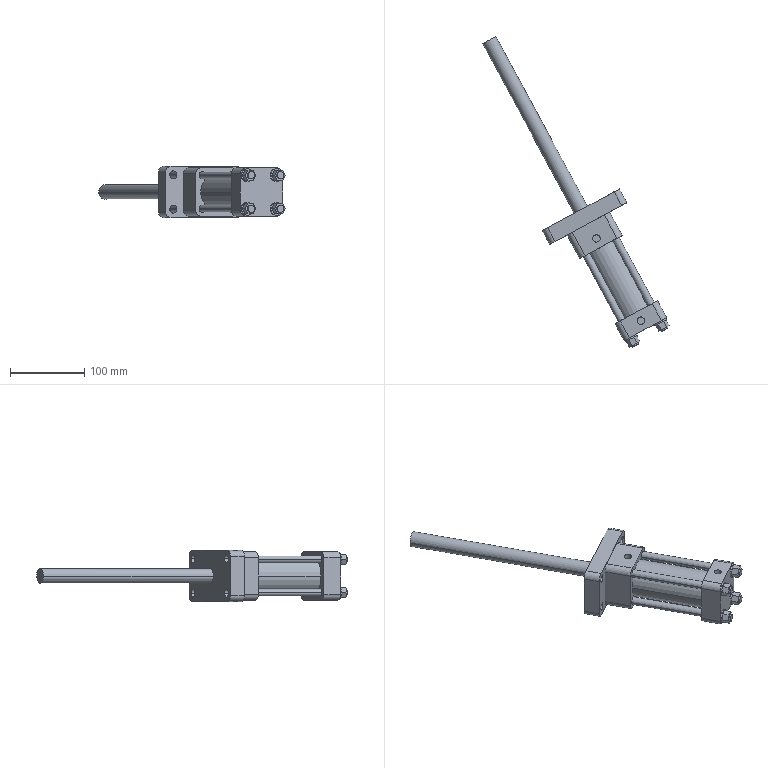Part | Creo | 1 solid | 108 faces | box 251.432 x 419.052 x 69 mm | volume 733506 mm3 | plane 56 | cylinder 52 | commonest cylinder face diameters 10 x20 16 x12 11 x8 18 x8 20 x2 50 x2